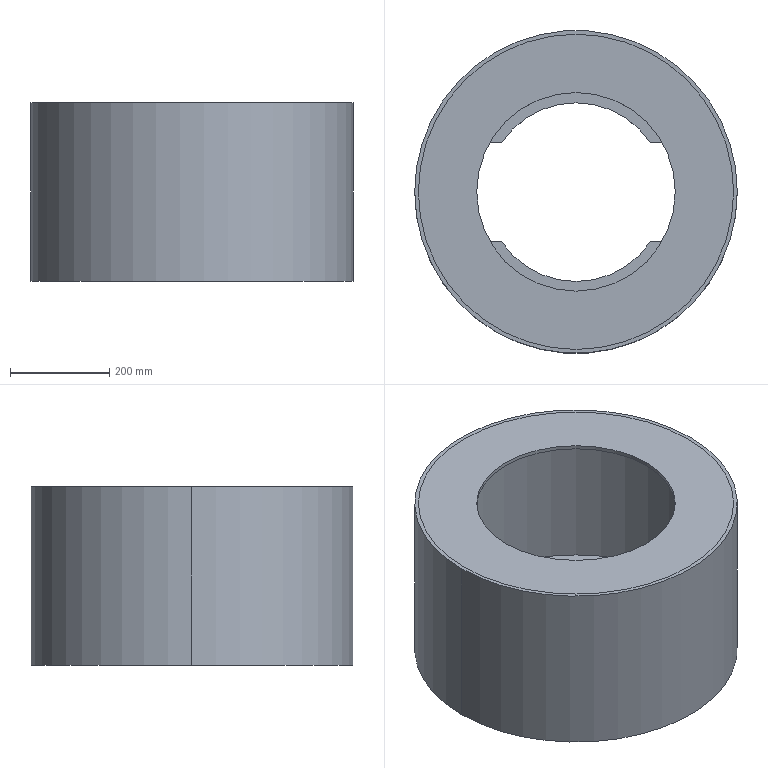Part | SolidWorks | features ICE 3, Cut 1, Extrusion 1 | 2 solids | 29 faces | box 650 x 650 x 360 mm | volume 8402293 mm3 | cylinder 18 | plane 11 | commonest cylinder face diameters 11 x8 635 x4 360 x2 400 x2 650 x2
STEP:
#1=CARTESIAN_POINT('',(108.,-177.535,7.5));
#2=VERTEX_POINT('',#1);
#3=CARTESIAN_POINT('',(97.,-177.535,7.5));
#4=VERTEX_POINT('',#3);
#5=CARTESIAN_POINT('',(102.5,-177.535,7.5));
#6=DIRECTION('',(0.,0.,-1.));
#7=DIRECTION('',(-1.,0.,0.));
#8=AXIS2_PLACEMENT_3D('',#5,#6,#7);
#9=CIRCLE('',#8,5.5);
#10=EDGE_CURVE('',#2,#4,#9,.T.);
#11=ORIENTED_EDGE('',*,*,#10,.F.);
#12=CARTESIAN_POINT('',(108.,-177.535,0.));
#13=VERTEX_POINT('',#12);
#14=CARTESIAN_POINT('',(108.,-177.535,10.));
#15=DIRECTION('',(0.,0.,-1.));
#16=VECTOR('',#15,1000.);
#17=LINE('',#14,#16);
#18=EDGE_CURVE('',#2,#13,#17,.T.);
#19=ORIENTED_EDGE('',*,*,#18,.T.);
#20=CARTESIAN_POINT('',(97.,-177.535,0.));
#21=VERTEX_POINT('',#20);
#22=CARTESIAN_POINT('',(102.5,-177.535,0.));
#23=DIRECTION('',(0.,0.,-1.));
#24=DIRECTION('',(-1.,0.,0.));
#25=AXIS2_PLACEMENT_3D('',#22,#23,#24);
#26=CIRCLE('',#25,5.5);
#27=EDGE_CURVE('',#13,#21,#26,.T.);
#28=ORIENTED_EDGE('',*,*,#27,.T.);
#29=CARTESIAN_POINT('',(97.,-177.535,10.));
#30=DIRECTION('',(0.,0.,-1.));
#31=VECTOR('',#30,1000.);
#32=LINE('',#29,#31);
#33=EDGE_CURVE('',#4,#21,#32,.T.);
#34=ORIENTED_EDGE('',*,*,#33,.F.);
#35=EDGE_LOOP('',(#11,#19,#28,#34));
#36=FACE_OUTER_BOUND('',#35,.T.);
#37=CARTESIAN_POINT('',(102.5,-177.535,10.));
#38=DIRECTION('',(0.,0.,-1.));
#39=DIRECTION('',(-1.,0.,0.));
#40=AXIS2_PLACEMENT_3D('',#37,#38,#39);
#41=CYLINDRICAL_SURFACE('',#40,5.5);
#42=ADVANCED_FACE('',(#36),#41,.F.);
#43=CARTESIAN_POINT('',(-97.,-177.535,7.5));
#44=VERTEX_POINT('',#43);
#45=CARTESIAN_POINT('',(-108.,-177.535,7.5));
#46=VERTEX_POINT('',#45);
#47=CARTESIAN_POINT('',(-102.5,-177.535,7.5));
#48=DIRECTION('',(0.,0.,-1.));
#49=DIRECTION('',(-1.,0.,0.));
#50=AXIS2_PLACEMENT_3D('',#47,#48,#49);
#51=CIRCLE('',#50,5.5);
#52=EDGE_CURVE('',#44,#46,#51,.T.);
#53=ORIENTED_EDGE('',*,*,#52,.F.);
#54=CARTESIAN_POINT('',(-97.,-177.535,0.));
#55=VERTEX_POINT('',#54);
#56=CARTESIAN_POINT('',(-97.,-177.535,10.));
#57=DIRECTION('',(0.,0.,-1.));
#58=VECTOR('',#57,1000.);
#59=LINE('',#56,#58);
#60=EDGE_CURVE('',#44,#55,#59,.T.);
#61=ORIENTED_EDGE('',*,*,#60,.T.);
#62=CARTESIAN_POINT('',(-108.,-177.535,0.));
#63=VERTEX_POINT('',#62);
#64=CARTESIAN_POINT('',(-102.5,-177.535,0.));
#65=DIRECTION('',(0.,0.,-1.));
#66=DIRECTION('',(-1.,0.,0.));
#67=AXIS2_PLACEMENT_3D('',#64,#65,#66);
#68=CIRCLE('',#67,5.5);
#69=EDGE_CURVE('',#55,#63,#68,.T.);
#70=ORIENTED_EDGE('',*,*,#69,.T.);
#71=CARTESIAN_POINT('',(-108.,-177.535,10.));
#72=DIRECTION('',(0.,0.,-1.));
#73=VECTOR('',#72,1000.);
#74=LINE('',#71,#73);
#75=EDGE_CURVE('',#46,#63,#74,.T.);
#76=ORIENTED_EDGE('',*,*,#75,.F.);
#77=EDGE_LOOP('',(#53,#61,#70,#76));
#78=FACE_OUTER_BOUND('',#77,.T.);
#79=CARTESIAN_POINT('',(-102.5,-177.535,10.));
#80=DIRECTION('',(0.,0.,-1.));
#81=DIRECTION('',(-1.,0.,0.));
#82=AXIS2_PLACEMENT_3D('',#79,#80,#81);
#83=CYLINDRICAL_SURFACE('',#82,5.5);
#84=ADVANCED_FACE('',(#78),#83,.F.);
#85=CARTESIAN_POINT('',(-97.,177.535,7.5));
#86=VERTEX_POINT('',#85);
#87=CARTESIAN_POINT('',(-108.,177.535,7.5));
#88=VERTEX_POINT('',#87);
#89=CARTESIAN_POINT('',(-102.5,177.535,7.5));
#90=DIRECTION('',(0.,0.,-1.));
#91=DIRECTION('',(-1.,0.,0.));
#92=AXIS2_PLACEMENT_3D('',#89,#90,#91);
#93=CIRCLE('',#92,5.5);
#94=EDGE_CURVE('',#86,#88,#93,.T.);
#95=ORIENTED_EDGE('',*,*,#94,.F.);
#96=CARTESIAN_POINT('',(-97.,177.535,0.));
#97=VERTEX_POINT('',#96);
#98=CARTESIAN_POINT('',(-97.,177.535,10.));
#99=DIRECTION('',(0.,0.,-1.));
#100=VECTOR('',#99,1000.);
#101=LINE('',#98,#100);
#102=EDGE_CURVE('',#86,#97,#101,.T.);
#103=ORIENTED_EDGE('',*,*,#102,.T.);
#104=CARTESIAN_POINT('',(-108.,177.535,0.));
#105=VERTEX_POINT('',#104);
#106=CARTESIAN_POINT('',(-102.5,177.535,0.));
#107=DIRECTION('',(0.,0.,-1.));
#108=DIRECTION('',(-1.,0.,0.));
#109=AXIS2_PLACEMENT_3D('',#106,#107,#108);
#110=CIRCLE('',#109,5.5);
#111=EDGE_CURVE('',#97,#105,#110,.T.);
#112=ORIENTED_EDGE('',*,*,#111,.T.);
#113=CARTESIAN_POINT('',(-108.,177.535,10.));
#114=DIRECTION('',(0.,0.,-1.));
#115=VECTOR('',#114,1000.);
#116=LINE('',#113,#115);
#117=EDGE_CURVE('',#88,#105,#116,.T.);
#118=ORIENTED_EDGE('',*,*,#117,.F.);
#119=EDGE_LOOP('',(#95,#103,#112,#118));
#120=FACE_OUTER_BOUND('',#119,.T.);
#121=CARTESIAN_POINT('',(-102.5,177.535,10.));
#122=DIRECTION('',(0.,0.,-1.));
#123=DIRECTION('',(-1.,0.,0.));
#124=AXIS2_PLACEMENT_3D('',#121,#122,#123);
#125=CYLINDRICAL_SURFACE('',#124,5.5);
#126=ADVANCED_FACE('',(#120),#125,.F.);
#127=CARTESIAN_POINT('',(108.,177.535,7.5));
#128=VERTEX_POINT('',#127);
#129=CARTESIAN_POINT('',(97.,177.535,7.5));
#130=VERTEX_POINT('',#129);
#131=CARTESIAN_POINT('',(102.5,177.535,7.5));
#132=DIRECTION('',(0.,0.,-1.));
#133=DIRECTION('',(-1.,0.,0.));
#134=AXIS2_PLACEMENT_3D('',#131,#132,#133);
#135=CIRCLE('',#134,5.5);
#136=EDGE_CURVE('',#128,#130,#135,.T.);
#137=ORIENTED_EDGE('',*,*,#136,.F.);
#138=CARTESIAN_POINT('',(108.,177.535,0.));
#139=VERTEX_POINT('',#138);
#140=CARTESIAN_POINT('',(108.,177.535,10.));
#141=DIRECTION('',(0.,0.,-1.));
#142=VECTOR('',#141,1000.);
#143=LINE('',#140,#142);
#144=EDGE_CURVE('',#128,#139,#143,.T.);
#145=ORIENTED_EDGE('',*,*,#144,.T.);
#146=CARTESIAN_POINT('',(97.,177.535,0.));
#147=VERTEX_POINT('',#146);
#148=CARTESIAN_POINT('',(102.5,177.535,0.));
#149=DIRECTION('',(0.,0.,-1.));
#150=DIRECTION('',(-1.,0.,0.));
#151=AXIS2_PLACEMENT_3D('',#148,#149,#150);
#152=CIRCLE('',#151,5.5);
#153=EDGE_CURVE('',#139,#147,#152,.T.);
#154=ORIENTED_EDGE('',*,*,#153,.T.);
#155=CARTESIAN_POINT('',(97.,177.535,10.));
#156=DIRECTION('',(0.,0.,-1.));
#157=VECTOR('',#156,1000.);
#158=LINE('',#155,#157);
#159=EDGE_CURVE('',#130,#147,#158,.T.);
#160=ORIENTED_EDGE('',*,*,#159,.F.);
#161=EDGE_LOOP('',(#137,#145,#154,#160));
#162=FACE_OUTER_BOUND('',#161,.T.);
#163=CARTESIAN_POINT('',(102.5,177.535,10.));
#164=DIRECTION('',(0.,0.,-1.));
#165=DIRECTION('',(-1.,0.,0.));
#166=AXIS2_PLACEMENT_3D('',#163,#164,#165);
#167=CYLINDRICAL_SURFACE('',#166,5.5);
#168=ADVANCED_FACE('',(#162),#167,.F.);
#169=CARTESIAN_POINT('',(-317.5,0.,360.));
#170=VERTEX_POINT('',#169);
#171=CARTESIAN_POINT('',(317.5,0.,360.));
#172=VERTEX_POINT('',#171);
#173=CARTESIAN_POINT('',(0.,0.,360.));
#174=DIRECTION('',(0.,0.,1.));
#175=DIRECTION('',(1.,0.,0.));
#176=AXIS2_PLACEMENT_3D('',#173,#174,#175);
#177=CIRCLE('',#176,317.5);
#178=EDGE_CURVE('',#170,#172,#177,.T.);
#179=ORIENTED_EDGE('',*,*,#178,.T.);
#180=CARTESIAN_POINT('',(317.5,0.,7.5));
#181=VERTEX_POINT('',#180);
#182=CARTESIAN_POINT('',(317.5,0.,367.5));
#183=DIRECTION('',(0.,0.,-1.));
#184=VECTOR('',#183,1000.);
#185=LINE('',#182,#184);
#186=EDGE_CURVE('',#172,#181,#185,.T.);
#187=ORIENTED_EDGE('',*,*,#186,.T.);
#188=CARTESIAN_POINT('',(-317.5,0.,7.5));
#189=VERTEX_POINT('',#188);
#190=CARTESIAN_POINT('',(0.,0.,7.5));
#191=DIRECTION('',(0.,0.,-1.));
#192=DIRECTION('',(-1.,0.,0.));
#193=AXIS2_PLACEMENT_3D('',#190,#191,#192);
#194=CIRCLE('',#193,317.5);
#195=EDGE_CURVE('',#181,#189,#194,.T.);
#196=ORIENTED_EDGE('',*,*,#195,.T.);
#197=CARTESIAN_POINT('',(-317.5,0.,367.5));
#198=DIRECTION('',(0.,0.,-1.));
#199=VECTOR('',#198,1000.);
#200=LINE('',#197,#199);
#201=EDGE_CURVE('',#170,#189,#200,.T.);
#202=ORIENTED_EDGE('',*,*,#201,.F.);
#203=EDGE_LOOP('',(#179,#187,#196,#202));
#204=FACE_OUTER_BOUND('',#203,.T.);
#205=CARTESIAN_POINT('',(0.,0.,367.5));
#206=DIRECTION('',(0.,0.,-1.));
#207=DIRECTION('',(-1.,0.,0.));
#208=AXIS2_PLACEMENT_3D('',#205,#206,#207);
#209=CYLINDRICAL_SURFACE('',#208,317.5);
#210=ADVANCED_FACE('',(#204),#209,.F.);
#211=CARTESIAN_POINT('',(325.,0.,360.));
#212=VERTEX_POINT('',#211);
#213=CARTESIAN_POINT('',(-325.,0.,360.));
#214=VERTEX_POINT('',#213);
#215=CARTESIAN_POINT('',(0.,0.,360.));
#216=DIRECTION('',(0.,0.,1.));
#217=DIRECTION('',(1.,0.,0.));
#218=AXIS2_PLACEMENT_3D('',#215,#216,#217);
#219=CIRCLE('',#218,325.);
#220=EDGE_CURVE('',#212,#214,#219,.T.);
#221=ORIENTED_EDGE('',*,*,#220,.F.);
#222=CARTESIAN_POINT('',(325.,0.,0.));
#223=VERTEX_POINT('',#222);
#224=CARTESIAN_POINT('',(325.,0.,360.));
#225=DIRECTION('',(0.,0.,-1.));
#226=VECTOR('',#225,1000.);
#227=LINE('',#224,#226);
#228=EDGE_CURVE('',#212,#223,#227,.T.);
#229=ORIENTED_EDGE('',*,*,#228,.T.);
#230=CARTESIAN_POINT('',(-325.,0.,0.));
#231=VERTEX_POINT('',#230);
#232=CARTESIAN_POINT('',(0.,0.,0.));
#233=DIRECTION('',(0.,0.,1.));
#234=DIRECTION('',(1.,0.,0.));
#235=AXIS2_PLACEMENT_3D('',#232,#233,#234);
#236=CIRCLE('',#235,325.);
#237=EDGE_CURVE('',#223,#231,#236,.T.);
#238=ORIENTED_EDGE('',*,*,#237,.T.);
#239=CARTESIAN_POINT('',(-325.,0.,360.));
#240=DIRECTION('',(0.,0.,-1.));
#241=VECTOR('',#240,1000.);
#242=LINE('',#239,#241);
#243=EDGE_CURVE('',#214,#231,#242,.T.);
#244=ORIENTED_EDGE('',*,*,#243,.F.);
#245=EDGE_LOOP('',(#221,#229,#238,#244));
#246=FACE_OUTER_BOUND('',#245,.T.);
#247=CARTESIAN_POINT('',(0.,0.,360.));
#248=DIRECTION('',(0.,0.,-1.));
#249=DIRECTION('',(-1.,0.,0.));
#250=AXIS2_PLACEMENT_3D('',#247,#248,#249);
#251=CYLINDRICAL_SURFACE('',#250,325.);
#252=ADVANCED_FACE('',(#246),#251,.T.);
#253=CARTESIAN_POINT('',(-149.666,100.,0.));
#254=VERTEX_POINT('',#253);
#255=CARTESIAN_POINT('',(149.666,100.,0.));
#256=VERTEX_POINT('',#255);
#257=CARTESIAN_POINT('',(0.,0.,0.));
#258=DIRECTION('',(0.,0.,-1.));
#259=DIRECTION('',(-1.,0.,0.));
#260=AXIS2_PLACEMENT_3D('',#257,#258,#259);
#261=CIRCLE('',#260,180.);
#262=EDGE_CURVE('',#254,#256,#261,.T.);
#263=ORIENTED_EDGE('',*,*,#262,.T.);
#264=CARTESIAN_POINT('',(149.666,100.,7.5));
#265=VERTEX_POINT('',#264);
#266=CARTESIAN_POINT('',(149.666,100.,360.));
#267=DIRECTION('',(0.,0.,1.));
#268=VECTOR('',#267,1000.);
#269=LINE('',#266,#268);
#270=EDGE_CURVE('',#256,#265,#269,.T.);
#271=ORIENTED_EDGE('',*,*,#270,.T.);
#272=CARTESIAN_POINT('',(-149.666,100.,7.5));
#273=VERTEX_POINT('',#272);
#274=CARTESIAN_POINT('',(0.,0.,7.5));
#275=DIRECTION('',(0.,0.,1.));
#276=DIRECTION('',(-1.,0.,0.));
#277=AXIS2_PLACEMENT_3D('',#274,#275,#276);
#278=CIRCLE('',#277,180.);
#279=EDGE_CURVE('',#265,#273,#278,.T.);
#280=ORIENTED_EDGE('',*,*,#279,.T.);
#281=CARTESIAN_POINT('',(-149.666,100.,360.));
#282=DIRECTION('',(0.,0.,-1.));
#283=VECTOR('',#282,1000.);
#284=LINE('',#281,#283);
#285=EDGE_CURVE('',#273,#254,#284,.T.);
#286=ORIENTED_EDGE('',*,*,#285,.T.);
#287=EDGE_LOOP('',(#263,#271,#280,#286));
#288=FACE_OUTER_BOUND('',#287,.T.);
#289=CARTESIAN_POINT('',(0.,0.,360.));
#290=DIRECTION('',(0.,0.,-1.));
#291=DIRECTION('',(-1.,0.,0.));
#292=AXIS2_PLACEMENT_3D('',#289,#290,#291);
#293=CYLINDRICAL_SURFACE('',#292,180.);
#294=ADVANCED_FACE('',(#288),#293,.F.);
#295=ORIENTED_EDGE('',*,*,#228,.F.);
#296=CARTESIAN_POINT('',(0.,0.,360.));
#297=DIRECTION('',(0.,0.,1.));
#298=DIRECTION('',(1.,0.,0.));
#299=AXIS2_PLACEMENT_3D('',#296,#297,#298);
#300=CIRCLE('',#299,325.);
#301=EDGE_CURVE('',#214,#212,#300,.T.);
#302=ORIENTED_EDGE('',*,*,#301,.F.);
#303=ORIENTED_EDGE('',*,*,#243,.T.);
#304=CARTESIAN_POINT('',(0.,0.,0.));
#305=DIRECTION('',(0.,0.,1.));
#306=DIRECTION('',(1.,0.,0.));
#307=AXIS2_PLACEMENT_3D('',#304,#305,#306);
#308=CIRCLE('',#307,325.);
#309=EDGE_CURVE('',#231,#223,#308,.T.);
#310=ORIENTED_EDGE('',*,*,#309,.T.);
#311=EDGE_LOOP('',(#295,#302,#303,#310));
#312=FACE_OUTER_BOUND('',#311,.T.);
#313=CARTESIAN_POINT('',(0.,0.,360.));
#314=DIRECTION('',(0.,0.,-1.));
#315=DIRECTION('',(-1.,0.,0.));
#316=AXIS2_PLACEMENT_3D('',#313,#314,#315);
#317=CYLINDRICAL_SURFACE('',#316,325.);
#318=ADVANCED_FACE('',(#312),#317,.T.);
#319=ORIENTED_EDGE('',*,*,#178,.F.);
#320=CARTESIAN_POINT('',(0.,0.,360.));
#321=DIRECTION('',(0.,0.,1.));
#322=DIRECTION('',(1.,0.,0.));
#323=AXIS2_PLACEMENT_3D('',#320,#321,#322);
#324=CIRCLE('',#323,317.5);
#325=EDGE_CURVE('',#172,#170,#324,.T.);
#326=ORIENTED_EDGE('',*,*,#325,.F.);
#327=EDGE_LOOP('',(#319,#326));
#328=FACE_BOUND('',#327,.T.);
#329=ORIENTED_EDGE('',*,*,#301,.T.);
#330=ORIENTED_EDGE('',*,*,#220,.T.);
#331=EDGE_LOOP('',(#329,#330));
#332=FACE_OUTER_BOUND('',#331,.T.);
#333=CARTESIAN_POINT('',(0.,0.,360.));
#334=DIRECTION('',(0.,0.,1.));
#335=DIRECTION('',(1.,0.,0.));
#336=AXIS2_PLACEMENT_3D('',#333,#334,#335);
#337=PLANE('',#336);
#338=ADVANCED_FACE('',(#328,#332),#337,.T.);
#339=CARTESIAN_POINT('',(102.5,-177.535,0.));
#340=DIRECTION('',(0.,0.,-1.));
#341=DIRECTION('',(-1.,0.,0.));
#342=AXIS2_PLACEMENT_3D('',#339,#340,#341);
#343=CIRCLE('',#342,5.5);
#344=EDGE_CURVE('',#21,#13,#343,.T.);
#345=ORIENTED_EDGE('',*,*,#344,.F.);
#346=ORIENTED_EDGE('',*,*,#27,.F.);
#347=EDGE_LOOP('',(#345,#346));
#348=FACE_BOUND('',#347,.T.);
#349=CARTESIAN_POINT('',(-102.5,-177.535,0.));
#350=DIRECTION('',(0.,0.,-1.));
#351=DIRECTION('',(-1.,0.,0.));
#352=AXIS2_PLACEMENT_3D('',#349,#350,#351);
#353=CIRCLE('',#352,5.5);
#354=EDGE_CURVE('',#63,#55,#353,.T.);
#355=ORIENTED_EDGE('',*,*,#354,.F.);
#356=ORIENTED_EDGE('',*,*,#69,.F.);
#357=EDGE_LOOP('',(#355,#356));
#358=FACE_BOUND('',#357,.T.);
#359=CARTESIAN_POINT('',(-102.5,177.535,0.));
#360=DIRECTION('',(0.,0.,-1.));
#361=DIRECTION('',(-1.,0.,0.));
#362=AXIS2_PLACEMENT_3D('',#359,#360,#361);
#363=CIRCLE('',#362,5.5);
#364=EDGE_CURVE('',#105,#97,#363,.T.);
#365=ORIENTED_EDGE('',*,*,#364,.F.);
#366=ORIENTED_EDGE('',*,*,#111,.F.);
#367=EDGE_LOOP('',(#365,#366));
#368=FACE_BOUND('',#367,.T.);
#369=CARTESIAN_POINT('',(102.5,177.535,0.));
#370=DIRECTION('',(0.,0.,-1.));
#371=DIRECTION('',(-1.,0.,0.));
#372=AXIS2_PLACEMENT_3D('',#369,#370,#371);
#373=CIRCLE('',#372,5.5);
#374=EDGE_CURVE('',#147,#139,#373,.T.);
#375=ORIENTED_EDGE('',*,*,#374,.F.);
#376=ORIENTED_EDGE('',*,*,#153,.F.);
#377=EDGE_LOOP('',(#375,#376));
#378=FACE_BOUND('',#377,.T.);
#379=ORIENTED_EDGE('',*,*,#262,.F.);
#380=CARTESIAN_POINT('',(-200.,100.,0.));
#381=VERTEX_POINT('',#380);
#382=CARTESIAN_POINT('',(200.,100.,0.));
#383=DIRECTION('',(1.,0.,0.));
#384=VECTOR('',#383,1000.);
#385=LINE('',#382,#384);
#386=EDGE_CURVE('',#381,#254,#385,.T.);
#387=ORIENTED_EDGE('',*,*,#386,.F.);
#388=CARTESIAN_POINT('',(-200.,-100.,0.));
#389=VERTEX_POINT('',#388);
#390=CARTESIAN_POINT('',(-200.,100.,0.));
#391=DIRECTION('',(0.,1.,0.));
#392=VECTOR('',#391,1000.);
#393=LINE('',#390,#392);
#394=EDGE_CURVE('',#389,#381,#393,.T.);
#395=ORIENTED_EDGE('',*,*,#394,.F.);
#396=CARTESIAN_POINT('',(-149.666,-100.,0.));
#397=VERTEX_POINT('',#396);
#398=CARTESIAN_POINT('',(200.,-100.,0.));
#399=DIRECTION('',(-1.,0.,0.));
#400=VECTOR('',#399,1000.);
#401=LINE('',#398,#400);
#402=EDGE_CURVE('',#397,#389,#401,.T.);
#403=ORIENTED_EDGE('',*,*,#402,.F.);
#404=CARTESIAN_POINT('',(149.666,-100.,0.));
#405=VERTEX_POINT('',#404);
#406=CARTESIAN_POINT('',(0.,0.,0.));
#407=DIRECTION('',(0.,0.,-1.));
#408=DIRECTION('',(-1.,0.,0.));
#409=AXIS2_PLACEMENT_3D('',#406,#407,#408);
#410=CIRCLE('',#409,180.);
#411=EDGE_CURVE('',#405,#397,#410,.T.);
#412=ORIENTED_EDGE('',*,*,#411,.F.);
#413=CARTESIAN_POINT('',(200.,-100.,0.));
#414=VERTEX_POINT('',#413);
#415=CARTESIAN_POINT('',(200.,-100.,0.));
#416=DIRECTION('',(-1.,0.,0.));
#417=VECTOR('',#416,1000.);
#418=LINE('',#415,#417);
#419=EDGE_CURVE('',#414,#405,#418,.T.);
#420=ORIENTED_EDGE('',*,*,#419,.F.);
#421=CARTESIAN_POINT('',(200.,100.,0.));
#422=VERTEX_POINT('',#421);
#423=CARTESIAN_POINT('',(200.,100.,0.));
#424=DIRECTION('',(0.,-1.,0.));
#425=VECTOR('',#424,1000.);
#426=LINE('',#423,#425);
#427=EDGE_CURVE('',#422,#414,#426,.T.);
#428=ORIENTED_EDGE('',*,*,#427,.F.);
#429=CARTESIAN_POINT('',(200.,100.,0.));
#430=DIRECTION('',(1.,0.,0.));
#431=VECTOR('',#430,1000.);
#432=LINE('',#429,#431);
#433=EDGE_CURVE('',#256,#422,#432,.T.);
#434=ORIENTED_EDGE('',*,*,#433,.F.);
#435=EDGE_LOOP('',(#379,#387,#395,#403,#412,#420,#428,#434));
#436=FACE_BOUND('',#435,.T.);
#437=ORIENTED_EDGE('',*,*,#309,.F.);
#438=ORIENTED_EDGE('',*,*,#237,.F.);
#439=EDGE_LOOP('',(#437,#438));
#440=FACE_OUTER_BOUND('',#439,.T.);
#441=CARTESIAN_POINT('',(0.,0.,0.));
#442=DIRECTION('',(0.,0.,1.));
#443=DIRECTION('',(1.,0.,0.));
#444=AXIS2_PLACEMENT_3D('',#441,#442,#443);
#445=PLANE('',#444);
#446=ADVANCED_FACE('',(#348,#358,#368,#378,#436,#440),#445,.F.);
#447=ORIENTED_EDGE('',*,*,#411,.T.);
#448=CARTESIAN_POINT('',(-149.666,-100.,7.5));
#449=VERTEX_POINT('',#448);
#450=CARTESIAN_POINT('',(-149.666,-100.,360.));
#451=DIRECTION('',(0.,0.,1.));
#452=VECTOR('',#451,1000.);
#453=LINE('',#450,#452);
#454=EDGE_CURVE('',#397,#449,#453,.T.);
#455=ORIENTED_EDGE('',*,*,#454,.T.);
#456=CARTESIAN_POINT('',(149.666,-100.,7.5));
#457=VERTEX_POINT('',#456);
#458=CARTESIAN_POINT('',(0.,0.,7.5));
#459=DIRECTION('',(0.,0.,1.));
#460=DIRECTION('',(-1.,0.,0.));
#461=AXIS2_PLACEMENT_3D('',#458,#459,#460);
#462=CIRCLE('',#461,180.);
#463=EDGE_CURVE('',#449,#457,#462,.T.);
#464=ORIENTED_EDGE('',*,*,#463,.T.);
#465=CARTESIAN_POINT('',(149.666,-100.,360.));
#466=DIRECTION('',(0.,0.,-1.));
#467=VECTOR('',#466,1000.);
#468=LINE('',#465,#467);
#469=EDGE_CURVE('',#457,#405,#468,.T.);
#470=ORIENTED_EDGE('',*,*,#469,.T.);
#471=EDGE_LOOP('',(#447,#455,#464,#470));
#472=FACE_OUTER_BOUND('',#471,.T.);
#473=CARTESIAN_POINT('',(0.,0.,360.));
#474=DIRECTION('',(0.,0.,-1.));
#475=DIRECTION('',(-1.,0.,0.));
#476=AXIS2_PLACEMENT_3D('',#473,#474,#475);
#477=CYLINDRICAL_SURFACE('',#476,180.);
#478=ADVANCED_FACE('',(#472),#477,.F.);
#479=CARTESIAN_POINT('',(102.5,-177.535,7.5));
#480=DIRECTION('',(0.,0.,-1.));
#481=DIRECTION('',(-1.,0.,0.));
#482=AXIS2_PLACEMENT_3D('',#479,#480,#481);
#483=CIRCLE('',#482,5.5);
#484=EDGE_CURVE('',#4,#2,#483,.T.);
#485=ORIENTED_EDGE('',*,*,#484,.T.);
#486=ORIENTED_EDGE('',*,*,#10,.T.);
#487=EDGE_LOOP('',(#485,#486));
#488=FACE_BOUND('',#487,.T.);
#489=CARTESIAN_POINT('',(-102.5,-177.535,7.5));
#490=DIRECTION('',(0.,0.,-1.));
#491=DIRECTION('',(-1.,0.,0.));
#492=AXIS2_PLACEMENT_3D('',#489,#490,#491);
#493=CIRCLE('',#492,5.5);
#494=EDGE_CURVE('',#46,#44,#493,.T.);
#495=ORIENTED_EDGE('',*,*,#494,.T.);
#496=ORIENTED_EDGE('',*,*,#52,.T.);
#497=EDGE_LOOP('',(#495,#496));
#498=FACE_BOUND('',#497,.T.);
#499=CARTESIAN_POINT('',(-102.5,177.535,7.5));
#500=DIRECTION('',(0.,0.,-1.));
#501=DIRECTION('',(-1.,0.,0.));
#502=AXIS2_PLACEMENT_3D('',#499,#500,#501);
#503=CIRCLE('',#502,5.5);
#504=EDGE_CURVE('',#88,#86,#503,.T.);
#505=ORIENTED_EDGE('',*,*,#504,.T.);
#506=ORIENTED_EDGE('',*,*,#94,.T.);
#507=EDGE_LOOP('',(#505,#506));
#508=FACE_BOUND('',#507,.T.);
#509=CARTESIAN_POINT('',(102.5,177.535,7.5));
#510=DIRECTION('',(0.,0.,-1.));
#511=DIRECTION('',(-1.,0.,0.));
#512=AXIS2_PLACEMENT_3D('',#509,#510,#511);
#513=CIRCLE('',#512,5.5);
#514=EDGE_CURVE('',#130,#128,#513,.T.);
#515=ORIENTED_EDGE('',*,*,#514,.T.);
#516=ORIENTED_EDGE('',*,*,#136,.T.);
#517=EDGE_LOOP('',(#515,#516));
#518=FACE_BOUND('',#517,.T.);
#519=CARTESIAN_POINT('',(0.,0.,7.5));
#520=DIRECTION('',(0.,0.,-1.));
#521=DIRECTION('',(-1.,0.,0.));
#522=AXIS2_PLACEMENT_3D('',#519,#520,#521);
#523=CIRCLE('',#522,317.5);
#524=EDGE_CURVE('',#189,#181,#523,.T.);
#525=ORIENTED_EDGE('',*,*,#524,.F.);
#526=ORIENTED_EDGE('',*,*,#195,.F.);
#527=EDGE_LOOP('',(#525,#526));
#528=FACE_OUTER_BOUND('',#527,.T.);
#529=ORIENTED_EDGE('',*,*,#279,.F.);
#530=CARTESIAN_POINT('',(200.,100.,7.5));
#531=VERTEX_POINT('',#530);
#532=CARTESIAN_POINT('',(0.,100.,7.5));
#533=DIRECTION('',(1.,0.,0.));
#534=VECTOR('',#533,1000.);
#535=LINE('',#532,#534);
#536=EDGE_CURVE('',#265,#531,#535,.T.);
#537=ORIENTED_EDGE('',*,*,#536,.T.);
#538=CARTESIAN_POINT('',(200.,-100.,7.5));
#539=VERTEX_POINT('',#538);
#540=CARTESIAN_POINT('',(200.,0.,7.5));
#541=DIRECTION('',(0.,-1.,0.));
#542=VECTOR('',#541,1000.);
#543=LINE('',#540,#542);
#544=EDGE_CURVE('',#531,#539,#543,.T.);
#545=ORIENTED_EDGE('',*,*,#544,.T.);
#546=CARTESIAN_POINT('',(0.,-100.,7.5));
#547=DIRECTION('',(-1.,0.,0.));
#548=VECTOR('',#547,1000.);
#549=LINE('',#546,#548);
#550=EDGE_CURVE('',#539,#457,#549,.T.);
#551=ORIENTED_EDGE('',*,*,#550,.T.);
#552=ORIENTED_EDGE('',*,*,#463,.F.);
#553=CARTESIAN_POINT('',(-200.,-100.,7.5));
#554=VERTEX_POINT('',#553);
#555=CARTESIAN_POINT('',(0.,-100.,7.5));
#556=DIRECTION('',(-1.,0.,0.));
#557=VECTOR('',#556,1000.);
#558=LINE('',#555,#557);
#559=EDGE_CURVE('',#449,#554,#558,.T.);
#560=ORIENTED_EDGE('',*,*,#559,.T.);
#561=CARTESIAN_POINT('',(-200.,100.,7.5));
#562=VERTEX_POINT('',#561);
#563=CARTESIAN_POINT('',(-200.,0.,7.5));
#564=DIRECTION('',(0.,1.,0.));
#565=VECTOR('',#564,1000.);
#566=LINE('',#563,#565);
#567=EDGE_CURVE('',#554,#562,#566,.T.);
#568=ORIENTED_EDGE('',*,*,#567,.T.);
#569=CARTESIAN_POINT('',(0.,100.,7.5));
#570=DIRECTION('',(1.,0.,0.));
#571=VECTOR('',#570,1000.);
#572=LINE('',#569,#571);
#573=EDGE_CURVE('',#562,#273,#572,.T.);
#574=ORIENTED_EDGE('',*,*,#573,.T.);
#575=EDGE_LOOP('',(#529,#537,#545,#551,#552,#560,#568,#574));
#576=FACE_BOUND('',#575,.T.);
#577=CARTESIAN_POINT('',(0.,0.,7.5));
#578=DIRECTION('',(0.,0.,-1.));
#579=DIRECTION('',(-1.,0.,0.));
#580=AXIS2_PLACEMENT_3D('',#577,#578,#579);
#581=PLANE('',#580);
#582=ADVANCED_FACE('',(#488,#498,#508,#518,#528,#576),#581,.F.);
#583=ORIENTED_EDGE('',*,*,#186,.F.);
#584=ORIENTED_EDGE('',*,*,#325,.T.);
#585=ORIENTED_EDGE('',*,*,#201,.T.);
#586=ORIENTED_EDGE('',*,*,#524,.T.);
#587=EDGE_LOOP('',(#583,#584,#585,#586));
#588=FACE_OUTER_BOUND('',#587,.T.);
#589=CARTESIAN_POINT('',(0.,0.,367.5));
#590=DIRECTION('',(0.,0.,-1.));
#591=DIRECTION('',(-1.,0.,0.));
#592=AXIS2_PLACEMENT_3D('',#589,#590,#591);
#593=CYLINDRICAL_SURFACE('',#592,317.5);
#594=ADVANCED_FACE('',(#588),#593,.F.);
#595=ORIENTED_EDGE('',*,*,#402,.T.);
#596=CARTESIAN_POINT('',(-200.,-100.,10.));
#597=DIRECTION('',(0.,0.,-1.));
#598=VECTOR('',#597,1000.);
#599=LINE('',#596,#598);
#600=EDGE_CURVE('',#554,#389,#599,.T.);
#601=ORIENTED_EDGE('',*,*,#600,.F.);
#602=ORIENTED_EDGE('',*,*,#559,.F.);
#603=ORIENTED_EDGE('',*,*,#454,.F.);
#604=EDGE_LOOP('',(#595,#601,#602,#603));
#605=FACE_OUTER_BOUND('',#604,.T.);
#606=CARTESIAN_POINT('',(200.,-100.,10.));
#607=DIRECTION('',(0.,-1.,0.));
#608=DIRECTION('',(0.,0.,-1.));
#609=AXIS2_PLACEMENT_3D('',#606,#607,#608);
#610=PLANE('',#609);
#611=ADVANCED_FACE('',(#605),#610,.F.);
#612=ORIENTED_EDGE('',*,*,#600,.T.);
#613=ORIENTED_EDGE('',*,*,#394,.T.);
#614=CARTESIAN_POINT('',(-200.,100.,10.));
#615=DIRECTION('',(0.,0.,-1.));
#616=VECTOR('',#615,1000.);
#617=LINE('',#614,#616);
#618=EDGE_CURVE('',#562,#381,#617,.T.);
#619=ORIENTED_EDGE('',*,*,#618,.F.);
#620=ORIENTED_EDGE('',*,*,#567,.F.);
#621=EDGE_LOOP('',(#612,#613,#619,#620));
#622=FACE_OUTER_BOUND('',#621,.T.);
#623=CARTESIAN_POINT('',(-200.,100.,10.));
#624=DIRECTION('',(-1.,0.,0.));
#625=DIRECTION('',(0.,0.,1.));
#626=AXIS2_PLACEMENT_3D('',#623,#624,#625);
#627=PLANE('',#626);
#628=ADVANCED_FACE('',(#622),#627,.F.);
#629=ORIENTED_EDGE('',*,*,#573,.F.);
#630=ORIENTED_EDGE('',*,*,#618,.T.);
#631=ORIENTED_EDGE('',*,*,#386,.T.);
#632=ORIENTED_EDGE('',*,*,#285,.F.);
#633=EDGE_LOOP('',(#629,#630,#631,#632));
#634=FACE_OUTER_BOUND('',#633,.T.);
#635=CARTESIAN_POINT('',(200.,100.,10.));
#636=DIRECTION('',(0.,1.,0.));
#637=DIRECTION('',(0.,0.,1.));
#638=AXIS2_PLACEMENT_3D('',#635,#636,#637);
#639=PLANE('',#638);
#640=ADVANCED_FACE('',(#634),#639,.F.);
#641=CARTESIAN_POINT('',(200.,100.,10.));
#642=DIRECTION('',(0.,0.,-1.));
#643=VECTOR('',#642,1000.);
#644=LINE('',#641,#643);
#645=EDGE_CURVE('',#531,#422,#644,.T.);
#646=ORIENTED_EDGE('',*,*,#645,.T.);
#647=ORIENTED_EDGE('',*,*,#427,.T.);
#648=CARTESIAN_POINT('',(200.,-100.,10.));
#649=DIRECTION('',(0.,0.,-1.));
#650=VECTOR('',#649,1000.);
#651=LINE('',#648,#650);
#652=EDGE_CURVE('',#539,#414,#651,.T.);
#653=ORIENTED_EDGE('',*,*,#652,.F.);
#654=ORIENTED_EDGE('',*,*,#544,.F.);
#655=EDGE_LOOP('',(#646,#647,#653,#654));
#656=FACE_OUTER_BOUND('',#655,.T.);
#657=CARTESIAN_POINT('',(200.,100.,10.));
#658=DIRECTION('',(1.,0.,0.));
#659=DIRECTION('',(0.,0.,-1.));
#660=AXIS2_PLACEMENT_3D('',#657,#658,#659);
#661=PLANE('',#660);
#662=ADVANCED_FACE('',(#656),#661,.F.);
#663=ORIENTED_EDGE('',*,*,#433,.T.);
#664=ORIENTED_EDGE('',*,*,#645,.F.);
#665=ORIENTED_EDGE('',*,*,#536,.F.);
#666=ORIENTED_EDGE('',*,*,#270,.F.);
#667=EDGE_LOOP('',(#663,#664,#665,#666));
#668=FACE_OUTER_BOUND('',#667,.T.);
#669=CARTESIAN_POINT('',(200.,100.,10.));
#670=DIRECTION('',(0.,1.,0.));
#671=DIRECTION('',(0.,0.,1.));
#672=AXIS2_PLACEMENT_3D('',#669,#670,#671);
#673=PLANE('',#672);
#674=ADVANCED_FACE('',(#668),#673,.F.);
#675=ORIENTED_EDGE('',*,*,#550,.F.);
#676=ORIENTED_EDGE('',*,*,#652,.T.);
#677=ORIENTED_EDGE('',*,*,#419,.T.);
#678=ORIENTED_EDGE('',*,*,#469,.F.);
#679=EDGE_LOOP('',(#675,#676,#677,#678));
#680=FACE_OUTER_BOUND('',#679,.T.);
#681=CARTESIAN_POINT('',(200.,-100.,10.));
#682=DIRECTION('',(0.,-1.,0.));
#683=DIRECTION('',(0.,0.,-1.));
#684=AXIS2_PLACEMENT_3D('',#681,#682,#683);
#685=PLANE('',#684);
#686=ADVANCED_FACE('',(#680),#685,.F.);
#687=ORIENTED_EDGE('',*,*,#144,.F.);
#688=ORIENTED_EDGE('',*,*,#514,.F.);
#689=ORIENTED_EDGE('',*,*,#159,.T.);
#690=ORIENTED_EDGE('',*,*,#374,.T.);
#691=EDGE_LOOP('',(#687,#688,#689,#690));
#692=FACE_OUTER_BOUND('',#691,.T.);
#693=CARTESIAN_POINT('',(102.5,177.535,10.));
#694=DIRECTION('',(0.,0.,-1.));
#695=DIRECTION('',(-1.,0.,0.));
#696=AXIS2_PLACEMENT_3D('',#693,#694,#695);
#697=CYLINDRICAL_SURFACE('',#696,5.5);
#698=ADVANCED_FACE('',(#692),#697,.F.);
#699=ORIENTED_EDGE('',*,*,#102,.F.);
#700=ORIENTED_EDGE('',*,*,#504,.F.);
#701=ORIENTED_EDGE('',*,*,#117,.T.);
#702=ORIENTED_EDGE('',*,*,#364,.T.);
#703=EDGE_LOOP('',(#699,#700,#701,#702));
#704=FACE_OUTER_BOUND('',#703,.T.);
#705=CARTESIAN_POINT('',(-102.5,177.535,10.));
#706=DIRECTION('',(0.,0.,-1.));
#707=DIRECTION('',(-1.,0.,0.));
#708=AXIS2_PLACEMENT_3D('',#705,#706,#707);
#709=CYLINDRICAL_SURFACE('',#708,5.5);
#710=ADVANCED_FACE('',(#704),#709,.F.);
#711=ORIENTED_EDGE('',*,*,#60,.F.);
#712=ORIENTED_EDGE('',*,*,#494,.F.);
#713=ORIENTED_EDGE('',*,*,#75,.T.);
#714=ORIENTED_EDGE('',*,*,#354,.T.);
#715=EDGE_LOOP('',(#711,#712,#713,#714));
#716=FACE_OUTER_BOUND('',#715,.T.);
#717=CARTESIAN_POINT('',(-102.5,-177.535,10.));
#718=DIRECTION('',(0.,0.,-1.));
#719=DIRECTION('',(-1.,0.,0.));
#720=AXIS2_PLACEMENT_3D('',#717,#718,#719);
#721=CYLINDRICAL_SURFACE('',#720,5.5);
#722=ADVANCED_FACE('',(#716),#721,.F.);
#723=ORIENTED_EDGE('',*,*,#18,.F.);
#724=ORIENTED_EDGE('',*,*,#484,.F.);
#725=ORIENTED_EDGE('',*,*,#33,.T.);
#726=ORIENTED_EDGE('',*,*,#344,.T.);
#727=EDGE_LOOP('',(#723,#724,#725,#726));
#728=FACE_OUTER_BOUND('',#727,.T.);
#729=CARTESIAN_POINT('',(102.5,-177.535,10.));
#730=DIRECTION('',(0.,0.,-1.));
#731=DIRECTION('',(-1.,0.,0.));
#732=AXIS2_PLACEMENT_3D('',#729,#730,#731);
#733=CYLINDRICAL_SURFACE('',#732,5.5);
#734=ADVANCED_FACE('',(#728),#733,.F.);
#735=CLOSED_SHELL('',(#42,#84,#126,#168,#210,#252,#294,#318,#338,#446,#478,#582,#594,#611,#628,#640,#662,#674,#686,#698,#710,#722,#734));
#736=MANIFOLD_SOLID_BREP('',#735);
#737=CARTESIAN_POINT('',(-200.,0.,352.5));
#738=VERTEX_POINT('',#737);
#739=CARTESIAN_POINT('',(200.,0.,352.5));
#740=VERTEX_POINT('',#739);
#741=CARTESIAN_POINT('',(0.,0.,352.5));
#742=DIRECTION('',(0.,0.,1.));
#743=DIRECTION('',(1.,0.,0.));
#744=AXIS2_PLACEMENT_3D('',#741,#742,#743);
#745=CIRCLE('',#744,200.);
#746=EDGE_CURVE('',#738,#740,#745,.T.);
#747=ORIENTED_EDGE('',*,*,#746,.F.);
#748=CARTESIAN_POINT('',(-200.,0.,360.));
#749=VERTEX_POINT('',#748);
#750=CARTESIAN_POINT('',(-200.,0.,352.5));
#751=DIRECTION('',(0.,0.,1.));
#752=VECTOR('',#751,1000.);
#753=LINE('',#750,#752);
#754=EDGE_CURVE('',#738,#749,#753,.T.);
#755=ORIENTED_EDGE('',*,*,#754,.T.);
#756=CARTESIAN_POINT('',(200.,0.,360.));
#757=VERTEX_POINT('',#756);
#758=CARTESIAN_POINT('',(0.,0.,360.));
#759=DIRECTION('',(0.,0.,1.));
#760=DIRECTION('',(1.,0.,0.));
#761=AXIS2_PLACEMENT_3D('',#758,#759,#760);
#762=CIRCLE('',#761,200.);
#763=EDGE_CURVE('',#749,#757,#762,.T.);
#764=ORIENTED_EDGE('',*,*,#763,.T.);
#765=CARTESIAN_POINT('',(200.,0.,352.5));
#766=DIRECTION('',(0.,0.,1.));
#767=VECTOR('',#766,1000.);
#768=LINE('',#765,#767);
#769=EDGE_CURVE('',#740,#757,#768,.T.);
#770=ORIENTED_EDGE('',*,*,#769,.F.);
#771=EDGE_LOOP('',(#747,#755,#764,#770));
#772=FACE_OUTER_BOUND('',#771,.T.);
#773=CARTESIAN_POINT('',(0.,0.,352.5));
#774=DIRECTION('',(0.,0.,1.));
#775=DIRECTION('',(1.,0.,0.));
#776=AXIS2_PLACEMENT_3D('',#773,#774,#775);
#777=CYLINDRICAL_SURFACE('',#776,200.);
#778=ADVANCED_FACE('',(#772),#777,.F.);
#779=CARTESIAN_POINT('',(317.5,0.,352.5));
#780=VERTEX_POINT('',#779);
#781=CARTESIAN_POINT('',(-317.5,0.,352.5));
#782=VERTEX_POINT('',#781);
#783=CARTESIAN_POINT('',(0.,0.,352.5));
#784=DIRECTION('',(0.,0.,1.));
#785=DIRECTION('',(1.,0.,0.));
#786=AXIS2_PLACEMENT_3D('',#783,#784,#785);
#787=CIRCLE('',#786,317.5);
#788=EDGE_CURVE('',#780,#782,#787,.T.);
#789=ORIENTED_EDGE('',*,*,#788,.T.);
#790=CARTESIAN_POINT('',(-317.5,0.,360.));
#791=VERTEX_POINT('',#790);
#792=CARTESIAN_POINT('',(-317.5,0.,352.5));
#793=DIRECTION('',(0.,0.,1.));
#794=VECTOR('',#793,1000.);
#795=LINE('',#792,#794);
#796=EDGE_CURVE('',#782,#791,#795,.T.);
#797=ORIENTED_EDGE('',*,*,#796,.T.);
#798=CARTESIAN_POINT('',(317.5,0.,360.));
#799=VERTEX_POINT('',#798);
#800=CARTESIAN_POINT('',(0.,0.,360.));
#801=DIRECTION('',(0.,0.,1.));
#802=DIRECTION('',(1.,0.,0.));
#803=AXIS2_PLACEMENT_3D('',#800,#801,#802);
#804=CIRCLE('',#803,317.5);
#805=EDGE_CURVE('',#799,#791,#804,.T.);
#806=ORIENTED_EDGE('',*,*,#805,.F.);
#807=CARTESIAN_POINT('',(317.5,0.,352.5));
#808=DIRECTION('',(0.,0.,1.));
#809=VECTOR('',#808,1000.);
#810=LINE('',#807,#809);
#811=EDGE_CURVE('',#780,#799,#810,.T.);
#812=ORIENTED_EDGE('',*,*,#811,.F.);
#813=EDGE_LOOP('',(#789,#797,#806,#812));
#814=FACE_OUTER_BOUND('',#813,.T.);
#815=CARTESIAN_POINT('',(0.,0.,352.5));
#816=DIRECTION('',(0.,0.,1.));
#817=DIRECTION('',(1.,0.,0.));
#818=AXIS2_PLACEMENT_3D('',#815,#816,#817);
#819=CYLINDRICAL_SURFACE('',#818,317.5);
#820=ADVANCED_FACE('',(#814),#819,.T.);
#821=ORIENTED_EDGE('',*,*,#796,.F.);
#822=CARTESIAN_POINT('',(0.,0.,352.5));
#823=DIRECTION('',(0.,0.,1.));
#824=DIRECTION('',(1.,0.,0.));
#825=AXIS2_PLACEMENT_3D('',#822,#823,#824);
#826=CIRCLE('',#825,317.5);
#827=EDGE_CURVE('',#782,#780,#826,.T.);
#828=ORIENTED_EDGE('',*,*,#827,.T.);
#829=ORIENTED_EDGE('',*,*,#811,.T.);
#830=CARTESIAN_POINT('',(0.,0.,360.));
#831=DIRECTION('',(0.,0.,1.));
#832=DIRECTION('',(1.,0.,0.));
#833=AXIS2_PLACEMENT_3D('',#830,#831,#832);
#834=CIRCLE('',#833,317.5);
#835=EDGE_CURVE('',#791,#799,#834,.T.);
#836=ORIENTED_EDGE('',*,*,#835,.F.);
#837=EDGE_LOOP('',(#821,#828,#829,#836));
#838=FACE_OUTER_BOUND('',#837,.T.);
#839=CARTESIAN_POINT('',(0.,0.,352.5));
#840=DIRECTION('',(0.,0.,1.));
#841=DIRECTION('',(1.,0.,0.));
#842=AXIS2_PLACEMENT_3D('',#839,#840,#841);
#843=CYLINDRICAL_SURFACE('',#842,317.5);
#844=ADVANCED_FACE('',(#838),#843,.T.);
#845=CARTESIAN_POINT('',(0.,0.,352.5));
#846=DIRECTION('',(0.,0.,1.));
#847=DIRECTION('',(1.,0.,0.));
#848=AXIS2_PLACEMENT_3D('',#845,#846,#847);
#849=CIRCLE('',#848,200.);
#850=EDGE_CURVE('',#740,#738,#849,.T.);
#851=ORIENTED_EDGE('',*,*,#850,.T.);
#852=ORIENTED_EDGE('',*,*,#746,.T.);
#853=EDGE_LOOP('',(#851,#852));
#854=FACE_BOUND('',#853,.T.);
#855=ORIENTED_EDGE('',*,*,#788,.F.);
#856=ORIENTED_EDGE('',*,*,#827,.F.);
#857=EDGE_LOOP('',(#855,#856));
#858=FACE_OUTER_BOUND('',#857,.T.);
#859=CARTESIAN_POINT('',(0.,0.,352.5));
#860=DIRECTION('',(0.,0.,1.));
#861=DIRECTION('',(1.,0.,0.));
#862=AXIS2_PLACEMENT_3D('',#859,#860,#861);
#863=PLANE('',#862);
#864=ADVANCED_FACE('',(#854,#858),#863,.F.);
#865=CARTESIAN_POINT('',(0.,0.,360.));
#866=DIRECTION('',(0.,0.,1.));
#867=DIRECTION('',(1.,0.,0.));
#868=AXIS2_PLACEMENT_3D('',#865,#866,#867);
#869=CIRCLE('',#868,200.);
#870=EDGE_CURVE('',#757,#749,#869,.T.);
#871=ORIENTED_EDGE('',*,*,#870,.F.);
#872=ORIENTED_EDGE('',*,*,#763,.F.);
#873=EDGE_LOOP('',(#871,#872));
#874=FACE_BOUND('',#873,.T.);
#875=ORIENTED_EDGE('',*,*,#805,.T.);
#876=ORIENTED_EDGE('',*,*,#835,.T.);
#877=EDGE_LOOP('',(#875,#876));
#878=FACE_OUTER_BOUND('',#877,.T.);
#879=CARTESIAN_POINT('',(0.,0.,360.));
#880=DIRECTION('',(0.,0.,1.));
#881=DIRECTION('',(1.,0.,0.));
#882=AXIS2_PLACEMENT_3D('',#879,#880,#881);
#883=PLANE('',#882);
#884=ADVANCED_FACE('',(#874,#878),#883,.T.);
#885=ORIENTED_EDGE('',*,*,#754,.F.);
#886=ORIENTED_EDGE('',*,*,#850,.F.);
#887=ORIENTED_EDGE('',*,*,#769,.T.);
#888=ORIENTED_EDGE('',*,*,#870,.T.);
#889=EDGE_LOOP('',(#885,#886,#887,#888));
#890=FACE_OUTER_BOUND('',#889,.T.);
#891=CARTESIAN_POINT('',(0.,0.,352.5));
#892=DIRECTION('',(0.,0.,1.));
#893=DIRECTION('',(1.,0.,0.));
#894=AXIS2_PLACEMENT_3D('',#891,#892,#893);
#895=CYLINDRICAL_SURFACE('',#894,200.);
#896=ADVANCED_FACE('',(#890),#895,.F.);
#897=CLOSED_SHELL('',(#778,#820,#844,#864,#884,#896));
#898=MANIFOLD_SOLID_BREP('',#897);
#899=CARTESIAN_POINT('',(0.,0.,0.));
#900=DIRECTION('',(0.,0.,1.));
#901=DIRECTION('',(1.,0.,0.));
#902=AXIS2_PLACEMENT_3D('',#899,#900,#901);
#903=(LENGTH_UNIT()NAMED_UNIT(*)SI_UNIT(.MILLI.,.METRE.));
#904=UNCERTAINTY_MEASURE_WITH_UNIT(LENGTH_MEASURE(0.00001),#903,'','');
#905=(NAMED_UNIT(*)PLANE_ANGLE_UNIT()SI_UNIT($,.RADIAN.));
#906=(NAMED_UNIT(*)SI_UNIT($,.STERADIAN.)SOLID_ANGLE_UNIT());
#907=(GEOMETRIC_REPRESENTATION_CONTEXT(3)GLOBAL_UNCERTAINTY_ASSIGNED_CONTEXT((#904))GLOBAL_UNIT_ASSIGNED_CONTEXT((#903,#905,#906))REPRESENTATION_CONTEXT('',''));
#908=ADVANCED_BREP_SHAPE_REPRESENTATION('',(#736,#898,#902),#907);